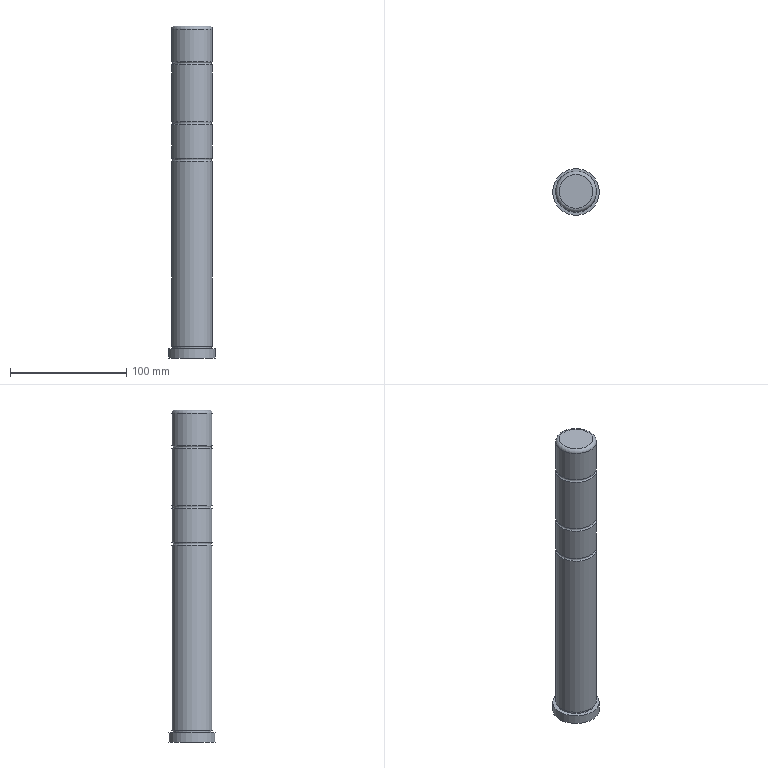Part | STEP file | 车灯-后视镜_id214_x_t | 1 solid | 18 faces | box 40 x 40 x 285 mm | volume 273765 mm3 | cylinder 8 | plane 5 | torus 4 | cone 1 | commonest cylinder face diameters 35 x4 8 x1 10 x1 33 x1 40 x1
STEP:
#1=CARTESIAN_POINT('',(-92.5,-185.,-248.914));
#2=VERTEX_POINT('',#1);
#3=CARTESIAN_POINT('',(-110.,-185.,-248.914));
#4=DIRECTION('',(0.,0.,1.));
#5=DIRECTION('',(1.,0.,0.));
#6=AXIS2_PLACEMENT_3D('',#3,#4,#5);
#7=CIRCLE('',#6,17.5);
#8=EDGE_CURVE('',#2,#2,#7,.T.);
#9=ORIENTED_EDGE('',*,*,#8,.T.);
#10=EDGE_LOOP('',(#9));
#11=FACE_BOUND('',#10,.T.);
#12=CARTESIAN_POINT('',(-127.5,-185.,-220.328));
#13=VERTEX_POINT('',#12);
#14=CARTESIAN_POINT('',(-110.,-185.,-220.328));
#15=DIRECTION('',(0.,0.,-1.));
#16=DIRECTION('',(-1.,0.,0.));
#17=AXIS2_PLACEMENT_3D('',#14,#15,#16);
#18=CIRCLE('',#17,17.5);
#19=EDGE_CURVE('',#13,#13,#18,.T.);
#20=ORIENTED_EDGE('',*,*,#19,.T.);
#21=EDGE_LOOP('',(#20));
#22=FACE_BOUND('',#21,.T.);
#23=CARTESIAN_POINT('',(-110.,-185.,-335.5));
#24=DIRECTION('',(0.,0.,1.));
#25=DIRECTION('',(-1.,0.,0.));
#26=AXIS2_PLACEMENT_3D('',#23,#24,#25);
#27=CYLINDRICAL_SURFACE('',#26,17.5);
#28=ADVANCED_FACE('',(#11,#22),#27,.T.);
#29=CARTESIAN_POINT('',(-127.5,-185.,-217.5));
#30=VERTEX_POINT('',#29);
#31=CARTESIAN_POINT('',(-110.,-185.,-217.5));
#32=DIRECTION('',(0.,0.,1.));
#33=DIRECTION('',(-1.,0.,0.));
#34=AXIS2_PLACEMENT_3D('',#31,#32,#33);
#35=CIRCLE('',#34,17.5);
#36=EDGE_CURVE('',#30,#30,#35,.T.);
#37=ORIENTED_EDGE('',*,*,#36,.T.);
#38=EDGE_LOOP('',(#37));
#39=FACE_BOUND('',#38,.T.);
#40=CARTESIAN_POINT('',(-127.5,-185.,-168.914));
#41=VERTEX_POINT('',#40);
#42=CARTESIAN_POINT('',(-110.,-185.,-168.914));
#43=DIRECTION('',(0.,0.,-1.));
#44=DIRECTION('',(-1.,0.,0.));
#45=AXIS2_PLACEMENT_3D('',#42,#43,#44);
#46=CIRCLE('',#45,17.5);
#47=EDGE_CURVE('',#41,#41,#46,.T.);
#48=ORIENTED_EDGE('',*,*,#47,.T.);
#49=EDGE_LOOP('',(#48));
#50=FACE_BOUND('',#49,.T.);
#51=CARTESIAN_POINT('',(-110.,-185.,-315.5));
#52=DIRECTION('',(0.,0.,1.));
#53=DIRECTION('',(-1.,0.,0.));
#54=AXIS2_PLACEMENT_3D('',#51,#52,#53);
#55=CYLINDRICAL_SURFACE('',#54,17.5);
#56=ADVANCED_FACE('',(#39,#50),#55,.T.);
#57=CARTESIAN_POINT('',(-92.5,-185.,-166.086));
#58=VERTEX_POINT('',#57);
#59=CARTESIAN_POINT('',(-110.,-185.,-166.086));
#60=DIRECTION('',(0.,0.,1.));
#61=DIRECTION('',(1.,0.,0.));
#62=AXIS2_PLACEMENT_3D('',#59,#60,#61);
#63=CIRCLE('',#62,17.5);
#64=EDGE_CURVE('',#58,#58,#63,.T.);
#65=ORIENTED_EDGE('',*,*,#64,.F.);
#66=EDGE_LOOP('',(#65));
#67=FACE_BOUND('',#66,.T.);
#68=ORIENTED_EDGE('',*,*,#47,.F.);
#69=EDGE_LOOP('',(#68));
#70=FACE_BOUND('',#69,.T.);
#71=CARTESIAN_POINT('',(-110.,-185.,-167.5));
#72=DIRECTION('',(0.,0.,1.));
#73=DIRECTION('',(-1.,0.,0.));
#74=AXIS2_PLACEMENT_3D('',#71,#72,#73);
#75=TOROIDAL_SURFACE('',#74,18.,1.5);
#76=ADVANCED_FACE('',(#67,#70),#75,.F.);
#77=CARTESIAN_POINT('',(-124.5,-185.,-135.5));
#78=VERTEX_POINT('',#77);
#79=CARTESIAN_POINT('',(-110.,-185.,-135.5));
#80=DIRECTION('',(0.,0.,-1.));
#81=DIRECTION('',(-1.,0.,0.));
#82=AXIS2_PLACEMENT_3D('',#79,#80,#81);
#83=CIRCLE('',#82,14.5);
#84=EDGE_CURVE('',#78,#78,#83,.T.);
#85=ORIENTED_EDGE('',*,*,#84,.F.);
#86=EDGE_LOOP('',(#85));
#87=FACE_OUTER_BOUND('',#86,.T.);
#88=CARTESIAN_POINT('',(-110.,-185.,-135.5));
#89=DIRECTION('',(0.,0.,1.));
#90=DIRECTION('',(-1.,0.,0.));
#91=AXIS2_PLACEMENT_3D('',#88,#89,#90);
#92=PLANE('',#91);
#93=ADVANCED_FACE('',(#87),#92,.T.);
#94=ORIENTED_EDGE('',*,*,#84,.T.);
#95=EDGE_LOOP('',(#94));
#96=FACE_BOUND('',#95,.T.);
#97=CARTESIAN_POINT('',(-127.5,-185.,-138.5));
#98=VERTEX_POINT('',#97);
#99=CARTESIAN_POINT('',(-110.,-185.,-138.5));
#100=DIRECTION('',(0.,0.,1.));
#101=DIRECTION('',(-1.,0.,0.));
#102=AXIS2_PLACEMENT_3D('',#99,#100,#101);
#103=CIRCLE('',#102,17.5);
#104=EDGE_CURVE('',#98,#98,#103,.T.);
#105=ORIENTED_EDGE('',*,*,#104,.T.);
#106=EDGE_LOOP('',(#105));
#107=FACE_BOUND('',#106,.T.);
#108=CARTESIAN_POINT('',(-110.,-185.,-138.5));
#109=DIRECTION('',(0.,0.,1.));
#110=DIRECTION('',(-1.,0.,0.));
#111=AXIS2_PLACEMENT_3D('',#108,#109,#110);
#112=TOROIDAL_SURFACE('',#111,14.5,3.);
#113=ADVANCED_FACE('',(#96,#107),#112,.T.);
#114=ORIENTED_EDGE('',*,*,#64,.T.);
#115=EDGE_LOOP('',(#114));
#116=FACE_BOUND('',#115,.T.);
#117=ORIENTED_EDGE('',*,*,#104,.F.);
#118=EDGE_LOOP('',(#117));
#119=FACE_BOUND('',#118,.T.);
#120=CARTESIAN_POINT('',(-110.,-185.,-315.5));
#121=DIRECTION('',(0.,0.,1.));
#122=DIRECTION('',(-1.,0.,0.));
#123=AXIS2_PLACEMENT_3D('',#120,#121,#122);
#124=CYLINDRICAL_SURFACE('',#123,17.5);
#125=ADVANCED_FACE('',(#116,#119),#124,.T.);
#126=ORIENTED_EDGE('',*,*,#36,.F.);
#127=EDGE_LOOP('',(#126));
#128=FACE_BOUND('',#127,.T.);
#129=ORIENTED_EDGE('',*,*,#19,.F.);
#130=EDGE_LOOP('',(#129));
#131=FACE_BOUND('',#130,.T.);
#132=CARTESIAN_POINT('',(-110.,-185.,-218.914));
#133=DIRECTION('',(0.,0.,1.));
#134=DIRECTION('',(-1.,0.,0.));
#135=AXIS2_PLACEMENT_3D('',#132,#133,#134);
#136=TOROIDAL_SURFACE('',#135,18.,1.5);
#137=ADVANCED_FACE('',(#128,#131),#136,.F.);
#138=ORIENTED_EDGE('',*,*,#8,.F.);
#139=EDGE_LOOP('',(#138));
#140=FACE_BOUND('',#139,.T.);
#141=CARTESIAN_POINT('',(-92.5,-185.,-251.743));
#142=VERTEX_POINT('',#141);
#143=CARTESIAN_POINT('',(-110.,-185.,-251.743));
#144=DIRECTION('',(0.,0.,-1.));
#145=DIRECTION('',(1.,0.,0.));
#146=AXIS2_PLACEMENT_3D('',#143,#144,#145);
#147=CIRCLE('',#146,17.5);
#148=EDGE_CURVE('',#142,#142,#147,.T.);
#149=ORIENTED_EDGE('',*,*,#148,.F.);
#150=EDGE_LOOP('',(#149));
#151=FACE_BOUND('',#150,.T.);
#152=CARTESIAN_POINT('',(-110.,-185.,-250.328));
#153=DIRECTION('',(0.,0.,1.));
#154=DIRECTION('',(-1.,0.,0.));
#155=AXIS2_PLACEMENT_3D('',#152,#153,#154);
#156=TOROIDAL_SURFACE('',#155,18.,1.5);
#157=ADVANCED_FACE('',(#140,#151),#156,.F.);
#158=CARTESIAN_POINT('',(-92.5,-185.,-410.5));
#159=VERTEX_POINT('',#158);
#160=CARTESIAN_POINT('',(-110.,-185.,-410.5));
#161=DIRECTION('',(0.,0.,1.));
#162=DIRECTION('',(1.,0.,0.));
#163=AXIS2_PLACEMENT_3D('',#160,#161,#162);
#164=CIRCLE('',#163,17.5);
#165=EDGE_CURVE('',#159,#159,#164,.T.);
#166=ORIENTED_EDGE('',*,*,#165,.T.);
#167=EDGE_LOOP('',(#166));
#168=FACE_BOUND('',#167,.T.);
#169=ORIENTED_EDGE('',*,*,#148,.T.);
#170=EDGE_LOOP('',(#169));
#171=FACE_BOUND('',#170,.T.);
#172=CARTESIAN_POINT('',(-110.,-185.,-405.5));
#173=DIRECTION('',(0.,0.,1.));
#174=DIRECTION('',(-1.,0.,0.));
#175=AXIS2_PLACEMENT_3D('',#172,#173,#174);
#176=CYLINDRICAL_SURFACE('',#175,17.5);
#177=ADVANCED_FACE('',(#168,#171),#176,.T.);
#178=CARTESIAN_POINT('',(-126.5,-185.,-410.5));
#179=VERTEX_POINT('',#178);
#180=CARTESIAN_POINT('',(-110.,-185.,-410.5));
#181=DIRECTION('',(0.,0.,-1.));
#182=DIRECTION('',(-1.,0.,0.));
#183=AXIS2_PLACEMENT_3D('',#180,#181,#182);
#184=CIRCLE('',#183,16.5);
#185=EDGE_CURVE('',#179,#179,#184,.T.);
#186=ORIENTED_EDGE('',*,*,#185,.T.);
#187=EDGE_LOOP('',(#186));
#188=FACE_BOUND('',#187,.T.);
#189=CARTESIAN_POINT('',(-126.5,-185.,-412.5));
#190=VERTEX_POINT('',#189);
#191=CARTESIAN_POINT('',(-110.,-185.,-412.5));
#192=DIRECTION('',(0.,0.,-1.));
#193=DIRECTION('',(-1.,0.,0.));
#194=AXIS2_PLACEMENT_3D('',#191,#192,#193);
#195=CIRCLE('',#194,16.5);
#196=EDGE_CURVE('',#190,#190,#195,.T.);
#197=ORIENTED_EDGE('',*,*,#196,.F.);
#198=EDGE_LOOP('',(#197));
#199=FACE_BOUND('',#198,.T.);
#200=CARTESIAN_POINT('',(-110.,-185.,-411.5));
#201=DIRECTION('',(0.,0.,1.));
#202=DIRECTION('',(-1.,0.,0.));
#203=AXIS2_PLACEMENT_3D('',#200,#201,#202);
#204=CYLINDRICAL_SURFACE('',#203,16.5);
#205=ADVANCED_FACE('',(#188,#199),#204,.T.);
#206=ORIENTED_EDGE('',*,*,#165,.F.);
#207=EDGE_LOOP('',(#206));
#208=FACE_BOUND('',#207,.T.);
#209=ORIENTED_EDGE('',*,*,#185,.F.);
#210=EDGE_LOOP('',(#209));
#211=FACE_BOUND('',#210,.T.);
#212=CARTESIAN_POINT('',(-110.,-185.,-410.5));
#213=DIRECTION('',(0.,0.,1.));
#214=DIRECTION('',(-1.,0.,0.));
#215=AXIS2_PLACEMENT_3D('',#212,#213,#214);
#216=PLANE('',#215);
#217=ADVANCED_FACE('',(#208,#211),#216,.F.);
#218=CARTESIAN_POINT('',(-115.,-185.,-420.5));
#219=VERTEX_POINT('',#218);
#220=CARTESIAN_POINT('',(-110.,-185.,-420.5));
#221=DIRECTION('',(0.,0.,-1.));
#222=DIRECTION('',(-1.,0.,0.));
#223=AXIS2_PLACEMENT_3D('',#220,#221,#222);
#224=CIRCLE('',#223,5.);
#225=EDGE_CURVE('',#219,#219,#224,.T.);
#226=ORIENTED_EDGE('',*,*,#225,.F.);
#227=EDGE_LOOP('',(#226));
#228=FACE_BOUND('',#227,.T.);
#229=CARTESIAN_POINT('',(-130.,-185.,-420.5));
#230=VERTEX_POINT('',#229);
#231=CARTESIAN_POINT('',(-110.,-185.,-420.5));
#232=DIRECTION('',(0.,0.,-1.));
#233=DIRECTION('',(-1.,0.,0.));
#234=AXIS2_PLACEMENT_3D('',#231,#232,#233);
#235=CIRCLE('',#234,20.);
#236=EDGE_CURVE('',#230,#230,#235,.T.);
#237=ORIENTED_EDGE('',*,*,#236,.T.);
#238=EDGE_LOOP('',(#237));
#239=FACE_BOUND('',#238,.T.);
#240=CARTESIAN_POINT('',(-110.,-185.,-420.5));
#241=DIRECTION('',(0.,0.,-1.));
#242=DIRECTION('',(1.,0.,0.));
#243=AXIS2_PLACEMENT_3D('',#240,#241,#242);
#244=PLANE('',#243);
#245=ADVANCED_FACE('',(#228,#239),#244,.T.);
#246=CARTESIAN_POINT('',(-90.,-185.,-412.5));
#247=VERTEX_POINT('',#246);
#248=CARTESIAN_POINT('',(-110.,-185.,-412.5));
#249=DIRECTION('',(0.,0.,1.));
#250=DIRECTION('',(1.,0.,0.));
#251=AXIS2_PLACEMENT_3D('',#248,#249,#250);
#252=CIRCLE('',#251,20.);
#253=EDGE_CURVE('',#247,#247,#252,.T.);
#254=ORIENTED_EDGE('',*,*,#253,.F.);
#255=EDGE_LOOP('',(#254));
#256=FACE_BOUND('',#255,.T.);
#257=ORIENTED_EDGE('',*,*,#236,.F.);
#258=EDGE_LOOP('',(#257));
#259=FACE_BOUND('',#258,.T.);
#260=CARTESIAN_POINT('',(-110.,-185.,-420.5));
#261=DIRECTION('',(0.,0.,1.));
#262=DIRECTION('',(-1.,0.,0.));
#263=AXIS2_PLACEMENT_3D('',#260,#261,#262);
#264=CYLINDRICAL_SURFACE('',#263,20.);
#265=ADVANCED_FACE('',(#256,#259),#264,.T.);
#266=ORIENTED_EDGE('',*,*,#253,.T.);
#267=EDGE_LOOP('',(#266));
#268=FACE_BOUND('',#267,.T.);
#269=ORIENTED_EDGE('',*,*,#196,.T.);
#270=EDGE_LOOP('',(#269));
#271=FACE_BOUND('',#270,.T.);
#272=CARTESIAN_POINT('',(-110.,-185.,-412.5));
#273=DIRECTION('',(0.,0.,1.));
#274=DIRECTION('',(-1.,0.,0.));
#275=AXIS2_PLACEMENT_3D('',#272,#273,#274);
#276=PLANE('',#275);
#277=ADVANCED_FACE('',(#268,#271),#276,.T.);
#278=CARTESIAN_POINT('',(-114.,-185.,-398.5));
#279=VERTEX_POINT('',#278);
#280=CARTESIAN_POINT('',(-110.,-185.,-398.5));
#281=DIRECTION('',(0.,0.,-1.));
#282=DIRECTION('',(-1.,0.,0.));
#283=AXIS2_PLACEMENT_3D('',#280,#281,#282);
#284=CIRCLE('',#283,4.);
#285=EDGE_CURVE('',#279,#279,#284,.T.);
#286=ORIENTED_EDGE('',*,*,#285,.T.);
#287=EDGE_LOOP('',(#286));
#288=FACE_BOUND('',#287,.T.);
#289=CARTESIAN_POINT('',(-110.,-185.,-396.097));
#290=VERTEX_POINT('',#289);
#291=VERTEX_LOOP('',#290);
#292=FACE_BOUND('',#291,.T.);
#293=CARTESIAN_POINT('',(-110.,-185.,-398.5));
#294=DIRECTION('',(0.,0.,-1.));
#295=DIRECTION('',(1.,0.,0.));
#296=AXIS2_PLACEMENT_3D('',#293,#294,#295);
#297=CONICAL_SURFACE('',#296,4.,59.);
#298=ADVANCED_FACE('',(#288,#292),#297,.F.);
#299=ORIENTED_EDGE('',*,*,#285,.F.);
#300=EDGE_LOOP('',(#299));
#301=FACE_BOUND('',#300,.T.);
#302=CARTESIAN_POINT('',(-114.,-185.,-400.5));
#303=VERTEX_POINT('',#302);
#304=CARTESIAN_POINT('',(-110.,-185.,-400.5));
#305=DIRECTION('',(0.,0.,-1.));
#306=DIRECTION('',(-1.,0.,0.));
#307=AXIS2_PLACEMENT_3D('',#304,#305,#306);
#308=CIRCLE('',#307,4.);
#309=EDGE_CURVE('',#303,#303,#308,.T.);
#310=ORIENTED_EDGE('',*,*,#309,.T.);
#311=EDGE_LOOP('',(#310));
#312=FACE_BOUND('',#311,.T.);
#313=CARTESIAN_POINT('',(-110.,-185.,-398.5));
#314=DIRECTION('',(0.,0.,1.));
#315=DIRECTION('',(-1.,0.,0.));
#316=AXIS2_PLACEMENT_3D('',#313,#314,#315);
#317=CYLINDRICAL_SURFACE('',#316,4.);
#318=ADVANCED_FACE('',(#301,#312),#317,.F.);
#319=ORIENTED_EDGE('',*,*,#309,.F.);
#320=EDGE_LOOP('',(#319));
#321=FACE_BOUND('',#320,.T.);
#322=CARTESIAN_POINT('',(-115.,-185.,-400.5));
#323=VERTEX_POINT('',#322);
#324=CARTESIAN_POINT('',(-110.,-185.,-400.5));
#325=DIRECTION('',(0.,0.,-1.));
#326=DIRECTION('',(-1.,0.,0.));
#327=AXIS2_PLACEMENT_3D('',#324,#325,#326);
#328=CIRCLE('',#327,5.);
#329=EDGE_CURVE('',#323,#323,#328,.T.);
#330=ORIENTED_EDGE('',*,*,#329,.T.);
#331=EDGE_LOOP('',(#330));
#332=FACE_BOUND('',#331,.T.);
#333=CARTESIAN_POINT('',(-110.,-185.,-400.5));
#334=DIRECTION('',(0.,0.,1.));
#335=DIRECTION('',(-1.,0.,0.));
#336=AXIS2_PLACEMENT_3D('',#333,#334,#335);
#337=PLANE('',#336);
#338=ADVANCED_FACE('',(#321,#332),#337,.F.);
#339=ORIENTED_EDGE('',*,*,#329,.F.);
#340=EDGE_LOOP('',(#339));
#341=FACE_BOUND('',#340,.T.);
#342=ORIENTED_EDGE('',*,*,#225,.T.);
#343=EDGE_LOOP('',(#342));
#344=FACE_BOUND('',#343,.T.);
#345=CARTESIAN_POINT('',(-110.,-185.,-420.5));
#346=DIRECTION('',(0.,0.,1.));
#347=DIRECTION('',(-1.,0.,0.));
#348=AXIS2_PLACEMENT_3D('',#345,#346,#347);
#349=CYLINDRICAL_SURFACE('',#348,5.);
#350=ADVANCED_FACE('',(#341,#344),#349,.F.);
#351=CLOSED_SHELL('',(#28,#56,#76,#93,#113,#125,#137,#157,#177,#205,#217,#245,#265,#277,#298,#318,#338,#350));
#352=MANIFOLD_SOLID_BREP('',#351);
#353=(LENGTH_UNIT()NAMED_UNIT(*)SI_UNIT(.MILLI.,.METRE.));
#354=UNCERTAINTY_MEASURE_WITH_UNIT(LENGTH_MEASURE(0.00002),#353,'','');
#355=(NAMED_UNIT(*)PLANE_ANGLE_UNIT()SI_UNIT($,.RADIAN.));
#356=PLANE_ANGLE_MEASURE_WITH_UNIT(PLANE_ANGLE_MEASURE(0.01745),#355);
#357=DIMENSIONAL_EXPONENTS(0.,0.,0.,0.,0.,0.,0.);
#358=(CONVERSION_BASED_UNIT('DEGREE',#356)NAMED_UNIT(#357)PLANE_ANGLE_UNIT());
#359=(NAMED_UNIT(*)SI_UNIT($,.STERADIAN.)SOLID_ANGLE_UNIT());
#360=(GEOMETRIC_REPRESENTATION_CONTEXT(3)GLOBAL_UNCERTAINTY_ASSIGNED_CONTEXT((#354))GLOBAL_UNIT_ASSIGNED_CONTEXT((#353,#358,#359))REPRESENTATION_CONTEXT('',''));
#361=ADVANCED_BREP_SHAPE_REPRESENTATION('',(#352),#360);